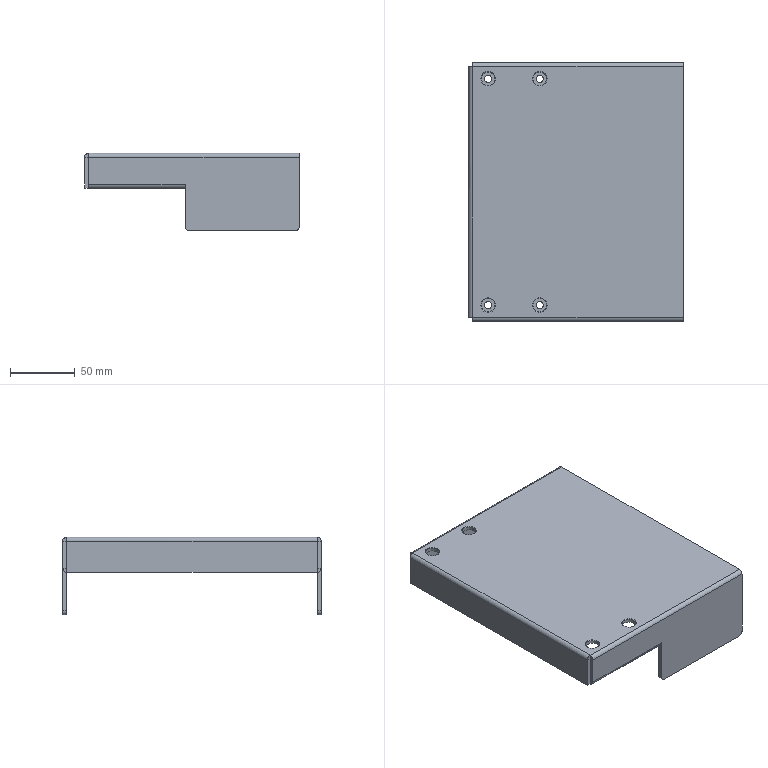Part | STEP file | 1 solid | 83 faces | box 166 x 200 x 60 mm | volume 160354 mm3 | plane 41 | cylinder 30 | cone 8 | spline 4 | commonest cylinder face diameters 5.5 x8 10.5 x8 0.2 x5 6.2 x5 6 x4